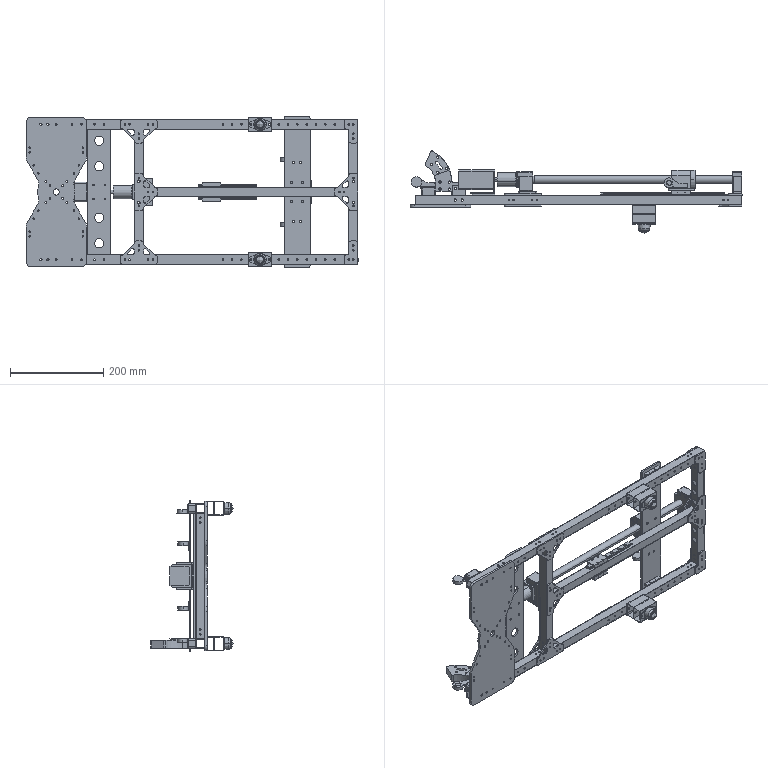Part | SolidWorks | 55 solids | 2224 faces | box 712 x 176.326 x 325 mm | volume 1220944 mm3 | cylinder 1519 | plane 665 | cone 20 | spline 20 | commonest cylinder face diameters 3.2 x516 5.5 x128 6 x113 3.5 x112 10 x110 5 x80